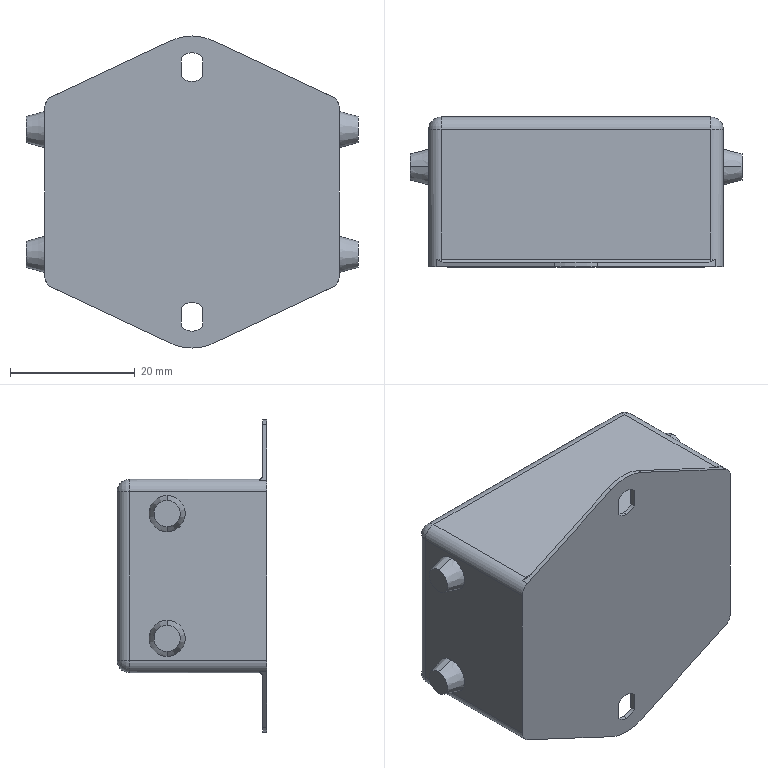Part | STEP file | Power line filter 3ACA5-W33 | 1 solid | 55 faces | box 53.2 x 24 x 50 mm | volume 35444 mm3 | plane 20 | cylinder 19 | cone 8 | sphere 4 | torus 4 | commonest cylinder face diameters 4 x8 4.6 x6 16 x3 1 x2